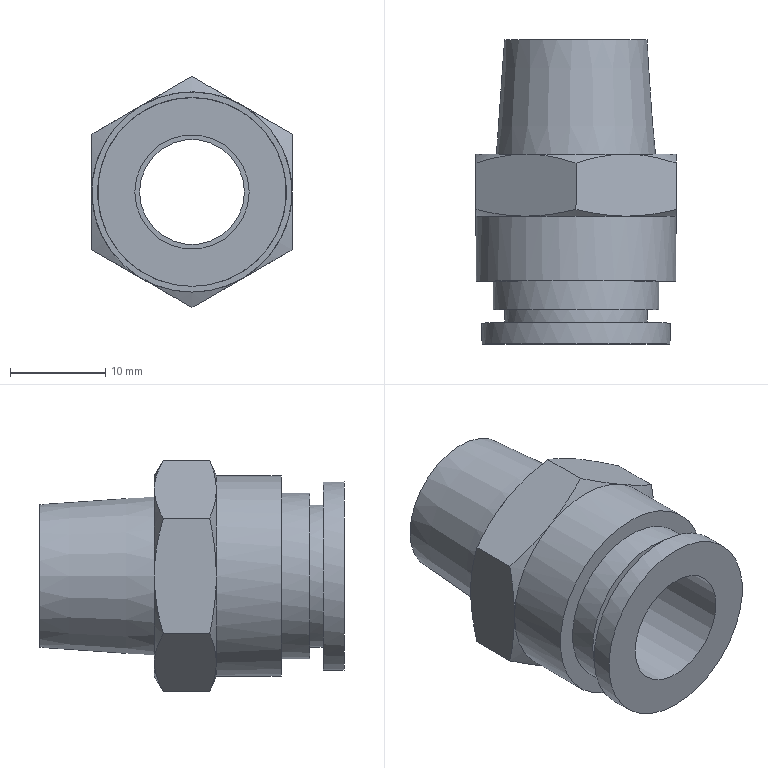Part | STEP file | 1_id114_xmt_txt | 1 solid | 32 faces | box 21 x 31.9 x 24.249 mm | volume 5376 mm3 | plane 13 | cone 13 | cylinder 6 | commonest cylinder face diameters 11 x1 12 x1 15 x1 17.4 x1 19.8 x1 21 x1
STEP:
#1=CARTESIAN_POINT('',(-25.5,-148.,61.));
#2=VERTEX_POINT('',#1);
#3=CARTESIAN_POINT('',(-18.,-148.,61.));
#4=DIRECTION('',(0.,-1.,0.));
#5=DIRECTION('',(-1.,0.,0.));
#6=AXIS2_PLACEMENT_3D('',#3,#4,#5);
#7=CIRCLE('',#6,7.5);
#8=EDGE_CURVE('',#2,#2,#7,.T.);
#9=ORIENTED_EDGE('',*,*,#8,.F.);
#10=EDGE_LOOP('',(#9));
#11=FACE_BOUND('',#10,.T.);
#12=CARTESIAN_POINT('',(-23.5,-148.,61.));
#13=VERTEX_POINT('',#12);
#14=CARTESIAN_POINT('',(-18.,-148.,61.));
#15=DIRECTION('',(0.,1.,0.));
#16=DIRECTION('',(-1.,0.,0.));
#17=AXIS2_PLACEMENT_3D('',#14,#15,#16);
#18=CIRCLE('',#17,5.5);
#19=EDGE_CURVE('',#13,#13,#18,.T.);
#20=ORIENTED_EDGE('',*,*,#19,.F.);
#21=EDGE_LOOP('',(#20));
#22=FACE_BOUND('',#21,.T.);
#23=CARTESIAN_POINT('',(-18.,-148.,61.));
#24=DIRECTION('',(0.,-1.,0.));
#25=DIRECTION('',(0.,0.,-1.));
#26=AXIS2_PLACEMENT_3D('',#23,#24,#25);
#27=PLANE('',#26);
#28=ADVANCED_FACE('',(#11,#22),#27,.F.);
#29=CARTESIAN_POINT('',(-9.65,-160.,61.));
#30=VERTEX_POINT('',#29);
#31=CARTESIAN_POINT('',(-18.,-160.,61.));
#32=DIRECTION('',(0.,-1.,0.));
#33=DIRECTION('',(1.,0.,0.));
#34=AXIS2_PLACEMENT_3D('',#31,#32,#33);
#35=CIRCLE('',#34,8.35);
#36=EDGE_CURVE('',#30,#30,#35,.T.);
#37=ORIENTED_EDGE('',*,*,#36,.F.);
#38=EDGE_LOOP('',(#37));
#39=FACE_BOUND('',#38,.T.);
#40=ORIENTED_EDGE('',*,*,#8,.T.);
#41=EDGE_LOOP('',(#40));
#42=FACE_BOUND('',#41,.T.);
#43=CARTESIAN_POINT('',(-18.,-154.,61.));
#44=DIRECTION('',(0.,-1.,0.));
#45=DIRECTION('',(-1.,0.,0.));
#46=AXIS2_PLACEMENT_3D('',#43,#44,#45);
#47=CONICAL_SURFACE('',#46,7.925,4.052);
#48=ADVANCED_FACE('',(#39,#42),#47,.T.);
#49=CARTESIAN_POINT('',(-23.25,-160.,70.093));
#50=VERTEX_POINT('',#49);
#51=CARTESIAN_POINT('',(-12.75,-160.,70.093));
#52=VERTEX_POINT('',#51);
#53=CARTESIAN_POINT('',(-18.,-160.,61.));
#54=DIRECTION('',(0.,1.,0.));
#55=DIRECTION('',(-0.5,0.,0.866));
#56=AXIS2_PLACEMENT_3D('',#53,#54,#55);
#57=CIRCLE('',#56,10.5);
#58=EDGE_CURVE('',#50,#52,#57,.T.);
#59=ORIENTED_EDGE('',*,*,#58,.T.);
#60=CARTESIAN_POINT('',(-7.5,-160.,61.));
#61=VERTEX_POINT('',#60);
#62=CARTESIAN_POINT('',(-18.,-160.,61.));
#63=DIRECTION('',(0.,1.,0.));
#64=DIRECTION('',(0.5,0.,0.866));
#65=AXIS2_PLACEMENT_3D('',#62,#63,#64);
#66=CIRCLE('',#65,10.5);
#67=EDGE_CURVE('',#52,#61,#66,.T.);
#68=ORIENTED_EDGE('',*,*,#67,.T.);
#69=CARTESIAN_POINT('',(-12.75,-160.,51.907));
#70=VERTEX_POINT('',#69);
#71=CARTESIAN_POINT('',(-18.,-160.,61.));
#72=DIRECTION('',(0.,1.,0.));
#73=DIRECTION('',(1.,0.,0.));
#74=AXIS2_PLACEMENT_3D('',#71,#72,#73);
#75=CIRCLE('',#74,10.5);
#76=EDGE_CURVE('',#61,#70,#75,.T.);
#77=ORIENTED_EDGE('',*,*,#76,.T.);
#78=CARTESIAN_POINT('',(-23.25,-160.,51.907));
#79=VERTEX_POINT('',#78);
#80=CARTESIAN_POINT('',(-18.,-160.,61.));
#81=DIRECTION('',(0.,1.,0.));
#82=DIRECTION('',(0.5,0.,-0.866));
#83=AXIS2_PLACEMENT_3D('',#80,#81,#82);
#84=CIRCLE('',#83,10.5);
#85=EDGE_CURVE('',#70,#79,#84,.T.);
#86=ORIENTED_EDGE('',*,*,#85,.T.);
#87=CARTESIAN_POINT('',(-28.5,-160.,61.));
#88=VERTEX_POINT('',#87);
#89=CARTESIAN_POINT('',(-18.,-160.,61.));
#90=DIRECTION('',(0.,1.,0.));
#91=DIRECTION('',(-0.5,0.,-0.866));
#92=AXIS2_PLACEMENT_3D('',#89,#90,#91);
#93=CIRCLE('',#92,10.5);
#94=EDGE_CURVE('',#79,#88,#93,.T.);
#95=ORIENTED_EDGE('',*,*,#94,.T.);
#96=CARTESIAN_POINT('',(-18.,-160.,61.));
#97=DIRECTION('',(0.,1.,0.));
#98=DIRECTION('',(-1.,0.,0.));
#99=AXIS2_PLACEMENT_3D('',#96,#97,#98);
#100=CIRCLE('',#99,10.5);
#101=EDGE_CURVE('',#88,#50,#100,.T.);
#102=ORIENTED_EDGE('',*,*,#101,.T.);
#103=EDGE_LOOP('',(#59,#68,#77,#86,#95,#102));
#104=FACE_BOUND('',#103,.T.);
#105=ORIENTED_EDGE('',*,*,#36,.T.);
#106=EDGE_LOOP('',(#105));
#107=FACE_BOUND('',#106,.T.);
#108=CARTESIAN_POINT('',(-18.,-160.,61.));
#109=DIRECTION('',(0.,-1.,0.));
#110=DIRECTION('',(0.,0.,-1.));
#111=AXIS2_PLACEMENT_3D('',#108,#109,#110);
#112=PLANE('',#111);
#113=ADVANCED_FACE('',(#104,#107),#112,.F.);
#114=ORIENTED_EDGE('',*,*,#101,.F.);
#115=CARTESIAN_POINT('',(-28.5,-160.938,67.062));
#116=VERTEX_POINT('',#115);
#117=CARTESIAN_POINT('',(-28.5,-160.,61.));
#118=CARTESIAN_POINT('',(-28.5,-160.,63.069));
#119=CARTESIAN_POINT('',(-28.5,-160.366,65.082));
#120=CARTESIAN_POINT('',(-28.5,-160.938,67.062));
#121=B_SPLINE_CURVE_WITH_KNOTS('',3,(#117,#118,#119,#120),.UNSPECIFIED.,.F.,.F.,(4,4),(0.,1.),.UNSPECIFIED.);
#122=EDGE_CURVE('',#88,#116,#121,.T.);
#123=ORIENTED_EDGE('',*,*,#122,.T.);
#124=CARTESIAN_POINT('',(-28.5,-160.938,67.062));
#125=CARTESIAN_POINT('',(-26.785,-160.366,68.052));
#126=CARTESIAN_POINT('',(-25.042,-160.,69.059));
#127=CARTESIAN_POINT('',(-23.25,-160.,70.093));
#128=B_SPLINE_CURVE_WITH_KNOTS('',3,(#124,#125,#126,#127),.UNSPECIFIED.,.F.,.F.,(4,4),(0.,1.),.UNSPECIFIED.);
#129=EDGE_CURVE('',#116,#50,#128,.T.);
#130=ORIENTED_EDGE('',*,*,#129,.T.);
#131=EDGE_LOOP('',(#114,#123,#130));
#132=FACE_OUTER_BOUND('',#131,.T.);
#133=CARTESIAN_POINT('',(-18.,-160.469,61.));
#134=DIRECTION('',(0.,-1.,0.));
#135=DIRECTION('',(-1.,0.,0.));
#136=AXIS2_PLACEMENT_3D('',#133,#134,#135);
#137=CONICAL_SURFACE('',#136,11.312,60.);
#138=ADVANCED_FACE('',(#132),#137,.T.);
#139=ORIENTED_EDGE('',*,*,#58,.F.);
#140=CARTESIAN_POINT('',(-18.,-160.938,73.124));
#141=VERTEX_POINT('',#140);
#142=CARTESIAN_POINT('',(-23.25,-160.,70.093));
#143=CARTESIAN_POINT('',(-21.458,-160.,71.128));
#144=CARTESIAN_POINT('',(-19.715,-160.366,72.134));
#145=CARTESIAN_POINT('',(-18.,-160.938,73.124));
#146=B_SPLINE_CURVE_WITH_KNOTS('',3,(#142,#143,#144,#145),.UNSPECIFIED.,.F.,.F.,(4,4),(0.,1.),.UNSPECIFIED.);
#147=EDGE_CURVE('',#50,#141,#146,.T.);
#148=ORIENTED_EDGE('',*,*,#147,.T.);
#149=CARTESIAN_POINT('',(-18.,-160.938,73.124));
#150=CARTESIAN_POINT('',(-16.285,-160.366,72.134));
#151=CARTESIAN_POINT('',(-14.542,-160.,71.128));
#152=CARTESIAN_POINT('',(-12.75,-160.,70.093));
#153=B_SPLINE_CURVE_WITH_KNOTS('',3,(#149,#150,#151,#152),.UNSPECIFIED.,.F.,.F.,(4,4),(0.,1.),.UNSPECIFIED.);
#154=EDGE_CURVE('',#141,#52,#153,.T.);
#155=ORIENTED_EDGE('',*,*,#154,.T.);
#156=EDGE_LOOP('',(#139,#148,#155));
#157=FACE_OUTER_BOUND('',#156,.T.);
#158=CARTESIAN_POINT('',(-18.,-160.469,61.));
#159=DIRECTION('',(0.,-1.,0.));
#160=DIRECTION('',(-1.,0.,0.));
#161=AXIS2_PLACEMENT_3D('',#158,#159,#160);
#162=CONICAL_SURFACE('',#161,11.312,60.);
#163=ADVANCED_FACE('',(#157),#162,.T.);
#164=ORIENTED_EDGE('',*,*,#67,.F.);
#165=CARTESIAN_POINT('',(-7.5,-160.938,67.062));
#166=VERTEX_POINT('',#165);
#167=CARTESIAN_POINT('',(-12.75,-160.,70.093));
#168=CARTESIAN_POINT('',(-10.958,-160.,69.059));
#169=CARTESIAN_POINT('',(-9.215,-160.366,68.052));
#170=CARTESIAN_POINT('',(-7.5,-160.938,67.062));
#171=B_SPLINE_CURVE_WITH_KNOTS('',3,(#167,#168,#169,#170),.UNSPECIFIED.,.F.,.F.,(4,4),(0.,1.),.UNSPECIFIED.);
#172=EDGE_CURVE('',#52,#166,#171,.T.);
#173=ORIENTED_EDGE('',*,*,#172,.T.);
#174=CARTESIAN_POINT('',(-7.5,-160.938,67.062));
#175=CARTESIAN_POINT('',(-7.5,-160.366,65.082));
#176=CARTESIAN_POINT('',(-7.5,-160.,63.069));
#177=CARTESIAN_POINT('',(-7.5,-160.,61.));
#178=B_SPLINE_CURVE_WITH_KNOTS('',3,(#174,#175,#176,#177),.UNSPECIFIED.,.F.,.F.,(4,4),(0.,1.),.UNSPECIFIED.);
#179=EDGE_CURVE('',#166,#61,#178,.T.);
#180=ORIENTED_EDGE('',*,*,#179,.T.);
#181=EDGE_LOOP('',(#164,#173,#180));
#182=FACE_OUTER_BOUND('',#181,.T.);
#183=CARTESIAN_POINT('',(-18.,-160.469,61.));
#184=DIRECTION('',(0.,-1.,0.));
#185=DIRECTION('',(-1.,0.,0.));
#186=AXIS2_PLACEMENT_3D('',#183,#184,#185);
#187=CONICAL_SURFACE('',#186,11.312,60.);
#188=ADVANCED_FACE('',(#182),#187,.T.);
#189=CARTESIAN_POINT('',(-18.,-165.798,73.124));
#190=VERTEX_POINT('',#189);
#191=CARTESIAN_POINT('',(-18.,-160.938,73.124));
#192=DIRECTION('',(0.,-1.,0.));
#193=VECTOR('',#192,1.);
#194=LINE('',#191,#193);
#195=EDGE_CURVE('',#141,#190,#194,.T.);
#196=ORIENTED_EDGE('',*,*,#195,.F.);
#197=ORIENTED_EDGE('',*,*,#147,.F.);
#198=ORIENTED_EDGE('',*,*,#129,.F.);
#199=CARTESIAN_POINT('',(-28.5,-165.798,67.062));
#200=VERTEX_POINT('',#199);
#201=CARTESIAN_POINT('',(-28.5,-160.938,67.062));
#202=DIRECTION('',(0.,-1.,0.));
#203=VECTOR('',#202,1.);
#204=LINE('',#201,#203);
#205=EDGE_CURVE('',#116,#200,#204,.T.);
#206=ORIENTED_EDGE('',*,*,#205,.T.);
#207=CARTESIAN_POINT('',(-23.25,-166.5,70.093));
#208=VERTEX_POINT('',#207);
#209=CARTESIAN_POINT('',(-23.25,-166.5,70.093));
#210=CARTESIAN_POINT('',(-25.023,-166.5,69.069));
#211=CARTESIAN_POINT('',(-26.77,-166.23,68.061));
#212=CARTESIAN_POINT('',(-28.5,-165.798,67.062));
#213=B_SPLINE_CURVE_WITH_KNOTS('',3,(#209,#210,#211,#212),.UNSPECIFIED.,.F.,.F.,(4,4),(0.,1.),.UNSPECIFIED.);
#214=EDGE_CURVE('',#208,#200,#213,.T.);
#215=ORIENTED_EDGE('',*,*,#214,.F.);
#216=CARTESIAN_POINT('',(-18.,-165.798,73.124));
#217=CARTESIAN_POINT('',(-19.73,-166.23,72.125));
#218=CARTESIAN_POINT('',(-21.477,-166.5,71.117));
#219=CARTESIAN_POINT('',(-23.25,-166.5,70.093));
#220=B_SPLINE_CURVE_WITH_KNOTS('',3,(#216,#217,#218,#219),.UNSPECIFIED.,.F.,.F.,(4,4),(0.,1.),.UNSPECIFIED.);
#221=EDGE_CURVE('',#190,#208,#220,.T.);
#222=ORIENTED_EDGE('',*,*,#221,.F.);
#223=EDGE_LOOP('',(#196,#197,#198,#206,#215,#222));
#224=FACE_OUTER_BOUND('',#223,.T.);
#225=CARTESIAN_POINT('',(-18.,-160.,73.124));
#226=DIRECTION('',(-0.5,0.,0.866));
#227=DIRECTION('',(0.866,0.,0.5));
#228=AXIS2_PLACEMENT_3D('',#225,#226,#227);
#229=PLANE('',#228);
#230=ADVANCED_FACE('',(#224),#229,.T.);
#231=CARTESIAN_POINT('',(-7.5,-166.5,61.));
#232=VERTEX_POINT('',#231);
#233=CARTESIAN_POINT('',(-7.5,-165.798,67.062));
#234=VERTEX_POINT('',#233);
#235=CARTESIAN_POINT('',(-7.5,-166.5,61.));
#236=CARTESIAN_POINT('',(-7.5,-166.5,63.048));
#237=CARTESIAN_POINT('',(-7.5,-166.23,65.064));
#238=CARTESIAN_POINT('',(-7.5,-165.798,67.062));
#239=B_SPLINE_CURVE_WITH_KNOTS('',3,(#235,#236,#237,#238),.UNSPECIFIED.,.F.,.F.,(4,4),(0.,1.),.UNSPECIFIED.);
#240=EDGE_CURVE('',#232,#234,#239,.T.);
#241=ORIENTED_EDGE('',*,*,#240,.T.);
#242=CARTESIAN_POINT('',(-12.75,-166.5,70.093));
#243=VERTEX_POINT('',#242);
#244=CARTESIAN_POINT('',(-7.5,-165.798,67.062));
#245=CARTESIAN_POINT('',(-9.23,-166.23,68.061));
#246=CARTESIAN_POINT('',(-10.977,-166.5,69.069));
#247=CARTESIAN_POINT('',(-12.75,-166.5,70.093));
#248=B_SPLINE_CURVE_WITH_KNOTS('',3,(#244,#245,#246,#247),.UNSPECIFIED.,.F.,.F.,(4,4),(0.,1.),.UNSPECIFIED.);
#249=EDGE_CURVE('',#234,#243,#248,.T.);
#250=ORIENTED_EDGE('',*,*,#249,.T.);
#251=CARTESIAN_POINT('',(-18.,-166.5,61.));
#252=DIRECTION('',(0.,-1.,0.));
#253=DIRECTION('',(1.,0.,0.));
#254=AXIS2_PLACEMENT_3D('',#251,#252,#253);
#255=CIRCLE('',#254,10.5);
#256=EDGE_CURVE('',#232,#243,#255,.T.);
#257=ORIENTED_EDGE('',*,*,#256,.F.);
#258=EDGE_LOOP('',(#241,#250,#257));
#259=FACE_OUTER_BOUND('',#258,.T.);
#260=CARTESIAN_POINT('',(-18.,-166.149,61.));
#261=DIRECTION('',(0.,1.,0.));
#262=DIRECTION('',(1.,0.,0.));
#263=AXIS2_PLACEMENT_3D('',#260,#261,#262);
#264=CONICAL_SURFACE('',#263,11.312,66.635);
#265=ADVANCED_FACE('',(#259),#264,.T.);
#266=CARTESIAN_POINT('',(-12.75,-166.5,70.093));
#267=CARTESIAN_POINT('',(-14.523,-166.5,71.117));
#268=CARTESIAN_POINT('',(-16.27,-166.23,72.125));
#269=CARTESIAN_POINT('',(-18.,-165.798,73.124));
#270=B_SPLINE_CURVE_WITH_KNOTS('',3,(#266,#267,#268,#269),.UNSPECIFIED.,.F.,.F.,(4,4),(0.,1.),.UNSPECIFIED.);
#271=EDGE_CURVE('',#243,#190,#270,.T.);
#272=ORIENTED_EDGE('',*,*,#271,.T.);
#273=ORIENTED_EDGE('',*,*,#221,.T.);
#274=CARTESIAN_POINT('',(-18.,-166.5,61.));
#275=DIRECTION('',(0.,-1.,0.));
#276=DIRECTION('',(0.,0.,1.));
#277=AXIS2_PLACEMENT_3D('',#274,#275,#276);
#278=CIRCLE('',#277,10.5);
#279=EDGE_CURVE('',#243,#208,#278,.T.);
#280=ORIENTED_EDGE('',*,*,#279,.F.);
#281=EDGE_LOOP('',(#272,#273,#280));
#282=FACE_OUTER_BOUND('',#281,.T.);
#283=CARTESIAN_POINT('',(-18.,-166.149,61.));
#284=DIRECTION('',(0.,1.,0.));
#285=DIRECTION('',(1.,0.,0.));
#286=AXIS2_PLACEMENT_3D('',#283,#284,#285);
#287=CONICAL_SURFACE('',#286,11.312,66.635);
#288=ADVANCED_FACE('',(#282),#287,.T.);
#289=ORIENTED_EDGE('',*,*,#214,.T.);
#290=CARTESIAN_POINT('',(-28.5,-166.5,61.));
#291=VERTEX_POINT('',#290);
#292=CARTESIAN_POINT('',(-28.5,-165.798,67.062));
#293=CARTESIAN_POINT('',(-28.5,-166.23,65.064));
#294=CARTESIAN_POINT('',(-28.5,-166.5,63.048));
#295=CARTESIAN_POINT('',(-28.5,-166.5,61.));
#296=B_SPLINE_CURVE_WITH_KNOTS('',3,(#292,#293,#294,#295),.UNSPECIFIED.,.F.,.F.,(4,4),(0.,1.),.UNSPECIFIED.);
#297=EDGE_CURVE('',#200,#291,#296,.T.);
#298=ORIENTED_EDGE('',*,*,#297,.T.);
#299=CARTESIAN_POINT('',(-18.,-166.5,61.));
#300=DIRECTION('',(0.,-1.,0.));
#301=DIRECTION('',(-0.5,0.,0.866));
#302=AXIS2_PLACEMENT_3D('',#299,#300,#301);
#303=CIRCLE('',#302,10.5);
#304=EDGE_CURVE('',#208,#291,#303,.T.);
#305=ORIENTED_EDGE('',*,*,#304,.F.);
#306=EDGE_LOOP('',(#289,#298,#305));
#307=FACE_OUTER_BOUND('',#306,.T.);
#308=CARTESIAN_POINT('',(-18.,-166.149,61.));
#309=DIRECTION('',(0.,1.,0.));
#310=DIRECTION('',(1.,0.,0.));
#311=AXIS2_PLACEMENT_3D('',#308,#309,#310);
#312=CONICAL_SURFACE('',#311,11.312,66.635);
#313=ADVANCED_FACE('',(#307),#312,.T.);
#314=CARTESIAN_POINT('',(-18.,-173.3,50.5));
#315=VERTEX_POINT('',#314);
#316=CARTESIAN_POINT('',(-18.,-173.3,61.));
#317=DIRECTION('',(0.,-1.,0.));
#318=DIRECTION('',(0.,0.,-1.));
#319=AXIS2_PLACEMENT_3D('',#316,#317,#318);
#320=CIRCLE('',#319,10.5);
#321=EDGE_CURVE('',#315,#315,#320,.T.);
#322=ORIENTED_EDGE('',*,*,#321,.F.);
#323=EDGE_LOOP('',(#322));
#324=FACE_BOUND('',#323,.T.);
#325=CARTESIAN_POINT('',(-12.75,-166.5,51.907));
#326=VERTEX_POINT('',#325);
#327=CARTESIAN_POINT('',(-18.,-166.5,61.));
#328=DIRECTION('',(0.,-1.,0.));
#329=DIRECTION('',(0.5,0.,-0.866));
#330=AXIS2_PLACEMENT_3D('',#327,#328,#329);
#331=CIRCLE('',#330,10.5);
#332=EDGE_CURVE('',#326,#232,#331,.T.);
#333=ORIENTED_EDGE('',*,*,#332,.T.);
#334=ORIENTED_EDGE('',*,*,#256,.T.);
#335=ORIENTED_EDGE('',*,*,#279,.T.);
#336=ORIENTED_EDGE('',*,*,#304,.T.);
#337=CARTESIAN_POINT('',(-23.25,-166.5,51.907));
#338=VERTEX_POINT('',#337);
#339=CARTESIAN_POINT('',(-18.,-166.5,61.));
#340=DIRECTION('',(0.,-1.,0.));
#341=DIRECTION('',(-1.,0.,0.));
#342=AXIS2_PLACEMENT_3D('',#339,#340,#341);
#343=CIRCLE('',#342,10.5);
#344=EDGE_CURVE('',#291,#338,#343,.T.);
#345=ORIENTED_EDGE('',*,*,#344,.T.);
#346=CARTESIAN_POINT('',(-18.,-166.5,61.));
#347=DIRECTION('',(0.,-1.,0.));
#348=DIRECTION('',(0.,0.,-1.));
#349=AXIS2_PLACEMENT_3D('',#346,#347,#348);
#350=CIRCLE('',#349,10.5);
#351=EDGE_CURVE('',#338,#326,#350,.T.);
#352=ORIENTED_EDGE('',*,*,#351,.T.);
#353=EDGE_LOOP('',(#333,#334,#335,#336,#345,#352));
#354=FACE_BOUND('',#353,.T.);
#355=CARTESIAN_POINT('',(-18.,-166.5,61.));
#356=DIRECTION('',(0.,1.,0.));
#357=DIRECTION('',(0.,0.,1.));
#358=AXIS2_PLACEMENT_3D('',#355,#356,#357);
#359=CYLINDRICAL_SURFACE('',#358,10.5);
#360=ADVANCED_FACE('',(#324,#354),#359,.T.);
#361=ORIENTED_EDGE('',*,*,#351,.F.);
#362=CARTESIAN_POINT('',(-18.,-165.798,48.876));
#363=VERTEX_POINT('',#362);
#364=CARTESIAN_POINT('',(-23.25,-166.5,51.907));
#365=CARTESIAN_POINT('',(-21.477,-166.5,50.883));
#366=CARTESIAN_POINT('',(-19.73,-166.23,49.875));
#367=CARTESIAN_POINT('',(-18.,-165.798,48.876));
#368=B_SPLINE_CURVE_WITH_KNOTS('',3,(#364,#365,#366,#367),.UNSPECIFIED.,.F.,.F.,(4,4),(0.,1.),.UNSPECIFIED.);
#369=EDGE_CURVE('',#338,#363,#368,.T.);
#370=ORIENTED_EDGE('',*,*,#369,.T.);
#371=CARTESIAN_POINT('',(-18.,-165.798,48.876));
#372=CARTESIAN_POINT('',(-16.27,-166.23,49.875));
#373=CARTESIAN_POINT('',(-14.523,-166.5,50.883));
#374=CARTESIAN_POINT('',(-12.75,-166.5,51.907));
#375=B_SPLINE_CURVE_WITH_KNOTS('',3,(#371,#372,#373,#374),.UNSPECIFIED.,.F.,.F.,(4,4),(0.,1.),.UNSPECIFIED.);
#376=EDGE_CURVE('',#363,#326,#375,.T.);
#377=ORIENTED_EDGE('',*,*,#376,.T.);
#378=EDGE_LOOP('',(#361,#370,#377));
#379=FACE_OUTER_BOUND('',#378,.T.);
#380=CARTESIAN_POINT('',(-18.,-166.149,61.));
#381=DIRECTION('',(0.,1.,0.));
#382=DIRECTION('',(1.,0.,0.));
#383=AXIS2_PLACEMENT_3D('',#380,#381,#382);
#384=CONICAL_SURFACE('',#383,11.312,66.635);
#385=ADVANCED_FACE('',(#379),#384,.T.);
#386=CARTESIAN_POINT('',(-7.5,-165.798,54.938));
#387=VERTEX_POINT('',#386);
#388=CARTESIAN_POINT('',(-12.75,-166.5,51.907));
#389=CARTESIAN_POINT('',(-10.977,-166.5,52.931));
#390=CARTESIAN_POINT('',(-9.23,-166.23,53.939));
#391=CARTESIAN_POINT('',(-7.5,-165.798,54.938));
#392=B_SPLINE_CURVE_WITH_KNOTS('',3,(#388,#389,#390,#391),.UNSPECIFIED.,.F.,.F.,(4,4),(0.,1.),.UNSPECIFIED.);
#393=EDGE_CURVE('',#326,#387,#392,.T.);
#394=ORIENTED_EDGE('',*,*,#393,.T.);
#395=CARTESIAN_POINT('',(-7.5,-165.798,54.938));
#396=CARTESIAN_POINT('',(-7.5,-166.23,56.936));
#397=CARTESIAN_POINT('',(-7.5,-166.5,58.952));
#398=CARTESIAN_POINT('',(-7.5,-166.5,61.));
#399=B_SPLINE_CURVE_WITH_KNOTS('',3,(#395,#396,#397,#398),.UNSPECIFIED.,.F.,.F.,(4,4),(0.,1.),.UNSPECIFIED.);
#400=EDGE_CURVE('',#387,#232,#399,.T.);
#401=ORIENTED_EDGE('',*,*,#400,.T.);
#402=ORIENTED_EDGE('',*,*,#332,.F.);
#403=EDGE_LOOP('',(#394,#401,#402));
#404=FACE_OUTER_BOUND('',#403,.T.);
#405=CARTESIAN_POINT('',(-18.,-166.149,61.));
#406=DIRECTION('',(0.,1.,0.));
#407=DIRECTION('',(1.,0.,0.));
#408=AXIS2_PLACEMENT_3D('',#405,#406,#407);
#409=CONICAL_SURFACE('',#408,11.312,66.635);
#410=ADVANCED_FACE('',(#404),#409,.T.);
#411=CARTESIAN_POINT('',(-28.5,-165.798,54.938));
#412=VERTEX_POINT('',#411);
#413=CARTESIAN_POINT('',(-28.5,-166.5,61.));
#414=CARTESIAN_POINT('',(-28.5,-166.5,58.952));
#415=CARTESIAN_POINT('',(-28.5,-166.23,56.936));
#416=CARTESIAN_POINT('',(-28.5,-165.798,54.938));
#417=B_SPLINE_CURVE_WITH_KNOTS('',3,(#413,#414,#415,#416),.UNSPECIFIED.,.F.,.F.,(4,4),(0.,1.),.UNSPECIFIED.);
#418=EDGE_CURVE('',#291,#412,#417,.T.);
#419=ORIENTED_EDGE('',*,*,#418,.T.);
#420=CARTESIAN_POINT('',(-28.5,-165.798,54.938));
#421=CARTESIAN_POINT('',(-26.77,-166.23,53.939));
#422=CARTESIAN_POINT('',(-25.023,-166.5,52.931));
#423=CARTESIAN_POINT('',(-23.25,-166.5,51.907));
#424=B_SPLINE_CURVE_WITH_KNOTS('',3,(#420,#421,#422,#423),.UNSPECIFIED.,.F.,.F.,(4,4),(0.,1.),.UNSPECIFIED.);
#425=EDGE_CURVE('',#412,#338,#424,.T.);
#426=ORIENTED_EDGE('',*,*,#425,.T.);
#427=ORIENTED_EDGE('',*,*,#344,.F.);
#428=EDGE_LOOP('',(#419,#426,#427));
#429=FACE_OUTER_BOUND('',#428,.T.);
#430=CARTESIAN_POINT('',(-18.,-166.149,61.));
#431=DIRECTION('',(0.,1.,0.));
#432=DIRECTION('',(1.,0.,0.));
#433=AXIS2_PLACEMENT_3D('',#430,#431,#432);
#434=CONICAL_SURFACE('',#433,11.312,66.635);
#435=ADVANCED_FACE('',(#429),#434,.T.);
#436=CARTESIAN_POINT('',(-18.,-160.938,48.876));
#437=VERTEX_POINT('',#436);
#438=CARTESIAN_POINT('',(-18.,-160.938,48.876));
#439=DIRECTION('',(0.,-1.,0.));
#440=VECTOR('',#439,1.);
#441=LINE('',#438,#440);
#442=EDGE_CURVE('',#437,#363,#441,.T.);
#443=ORIENTED_EDGE('',*,*,#442,.F.);
#444=CARTESIAN_POINT('',(-12.75,-160.,51.907));
#445=CARTESIAN_POINT('',(-14.542,-160.,50.872));
#446=CARTESIAN_POINT('',(-16.285,-160.366,49.866));
#447=CARTESIAN_POINT('',(-18.,-160.938,48.876));
#448=B_SPLINE_CURVE_WITH_KNOTS('',3,(#444,#445,#446,#447),.UNSPECIFIED.,.F.,.F.,(4,4),(0.,1.),.UNSPECIFIED.);
#449=EDGE_CURVE('',#70,#437,#448,.T.);
#450=ORIENTED_EDGE('',*,*,#449,.F.);
#451=CARTESIAN_POINT('',(-7.5,-160.938,54.938));
#452=VERTEX_POINT('',#451);
#453=CARTESIAN_POINT('',(-7.5,-160.938,54.938));
#454=CARTESIAN_POINT('',(-9.215,-160.366,53.948));
#455=CARTESIAN_POINT('',(-10.958,-160.,52.941));
#456=CARTESIAN_POINT('',(-12.75,-160.,51.907));
#457=B_SPLINE_CURVE_WITH_KNOTS('',3,(#453,#454,#455,#456),.UNSPECIFIED.,.F.,.F.,(4,4),(0.,1.),.UNSPECIFIED.);
#458=EDGE_CURVE('',#452,#70,#457,.T.);
#459=ORIENTED_EDGE('',*,*,#458,.F.);
#460=CARTESIAN_POINT('',(-7.5,-160.938,54.938));
#461=DIRECTION('',(0.,-1.,0.));
#462=VECTOR('',#461,1.);
#463=LINE('',#460,#462);
#464=EDGE_CURVE('',#452,#387,#463,.T.);
#465=ORIENTED_EDGE('',*,*,#464,.T.);
#466=ORIENTED_EDGE('',*,*,#393,.F.);
#467=ORIENTED_EDGE('',*,*,#376,.F.);
#468=EDGE_LOOP('',(#443,#450,#459,#465,#466,#467));
#469=FACE_OUTER_BOUND('',#468,.T.);
#470=CARTESIAN_POINT('',(-18.,-160.,48.876));
#471=DIRECTION('',(0.5,0.,-0.866));
#472=DIRECTION('',(0.,1.,0.));
#473=AXIS2_PLACEMENT_3D('',#470,#471,#472);
#474=PLANE('',#473);
#475=ADVANCED_FACE('',(#469),#474,.T.);
#476=ORIENTED_EDGE('',*,*,#464,.F.);
#477=CARTESIAN_POINT('',(-7.5,-160.,61.));
#478=CARTESIAN_POINT('',(-7.5,-160.,58.931));
#479=CARTESIAN_POINT('',(-7.5,-160.366,56.918));
#480=CARTESIAN_POINT('',(-7.5,-160.938,54.938));
#481=B_SPLINE_CURVE_WITH_KNOTS('',3,(#477,#478,#479,#480),.UNSPECIFIED.,.F.,.F.,(4,4),(0.,1.),.UNSPECIFIED.);
#482=EDGE_CURVE('',#61,#452,#481,.T.);
#483=ORIENTED_EDGE('',*,*,#482,.F.);
#484=ORIENTED_EDGE('',*,*,#179,.F.);
#485=CARTESIAN_POINT('',(-7.5,-160.938,67.062));
#486=DIRECTION('',(0.,-1.,0.));
#487=VECTOR('',#486,1.);
#488=LINE('',#485,#487);
#489=EDGE_CURVE('',#166,#234,#488,.T.);
#490=ORIENTED_EDGE('',*,*,#489,.T.);
#491=ORIENTED_EDGE('',*,*,#240,.F.);
#492=ORIENTED_EDGE('',*,*,#400,.F.);
#493=EDGE_LOOP('',(#476,#483,#484,#490,#491,#492));
#494=FACE_OUTER_BOUND('',#493,.T.);
#495=CARTESIAN_POINT('',(-7.5,-160.,54.938));
#496=DIRECTION('',(1.,0.,0.));
#497=DIRECTION('',(0.,0.,1.));
#498=AXIS2_PLACEMENT_3D('',#495,#496,#497);
#499=PLANE('',#498);
#500=ADVANCED_FACE('',(#494),#499,.T.);
#501=ORIENTED_EDGE('',*,*,#489,.F.);
#502=ORIENTED_EDGE('',*,*,#172,.F.);
#503=ORIENTED_EDGE('',*,*,#154,.F.);
#504=ORIENTED_EDGE('',*,*,#195,.T.);
#505=ORIENTED_EDGE('',*,*,#271,.F.);
#506=ORIENTED_EDGE('',*,*,#249,.F.);
#507=EDGE_LOOP('',(#501,#502,#503,#504,#505,#506));
#508=FACE_OUTER_BOUND('',#507,.T.);
#509=CARTESIAN_POINT('',(-7.5,-160.,67.062));
#510=DIRECTION('',(0.5,0.,0.866));
#511=DIRECTION('',(0.,1.,0.));
#512=AXIS2_PLACEMENT_3D('',#509,#510,#511);
#513=PLANE('',#512);
#514=ADVANCED_FACE('',(#508),#513,.T.);
#515=ORIENTED_EDGE('',*,*,#76,.F.);
#516=ORIENTED_EDGE('',*,*,#482,.T.);
#517=ORIENTED_EDGE('',*,*,#458,.T.);
#518=EDGE_LOOP('',(#515,#516,#517));
#519=FACE_OUTER_BOUND('',#518,.T.);
#520=CARTESIAN_POINT('',(-18.,-160.469,61.));
#521=DIRECTION('',(0.,-1.,0.));
#522=DIRECTION('',(-1.,0.,0.));
#523=AXIS2_PLACEMENT_3D('',#520,#521,#522);
#524=CONICAL_SURFACE('',#523,11.312,60.);
#525=ADVANCED_FACE('',(#519),#524,.T.);
#526=ORIENTED_EDGE('',*,*,#85,.F.);
#527=ORIENTED_EDGE('',*,*,#449,.T.);
#528=CARTESIAN_POINT('',(-18.,-160.938,48.876));
#529=CARTESIAN_POINT('',(-19.715,-160.366,49.866));
#530=CARTESIAN_POINT('',(-21.458,-160.,50.872));
#531=CARTESIAN_POINT('',(-23.25,-160.,51.907));
#532=B_SPLINE_CURVE_WITH_KNOTS('',3,(#528,#529,#530,#531),.UNSPECIFIED.,.F.,.F.,(4,4),(0.,1.),.UNSPECIFIED.);
#533=EDGE_CURVE('',#437,#79,#532,.T.);
#534=ORIENTED_EDGE('',*,*,#533,.T.);
#535=EDGE_LOOP('',(#526,#527,#534));
#536=FACE_OUTER_BOUND('',#535,.T.);
#537=CARTESIAN_POINT('',(-18.,-160.469,61.));
#538=DIRECTION('',(0.,-1.,0.));
#539=DIRECTION('',(-1.,0.,0.));
#540=AXIS2_PLACEMENT_3D('',#537,#538,#539);
#541=CONICAL_SURFACE('',#540,11.312,60.);
#542=ADVANCED_FACE('',(#536),#541,.T.);
#543=ORIENTED_EDGE('',*,*,#94,.F.);
#544=CARTESIAN_POINT('',(-28.5,-160.938,54.938));
#545=VERTEX_POINT('',#544);
#546=CARTESIAN_POINT('',(-23.25,-160.,51.907));
#547=CARTESIAN_POINT('',(-25.042,-160.,52.941));
#548=CARTESIAN_POINT('',(-26.785,-160.366,53.948));
#549=CARTESIAN_POINT('',(-28.5,-160.938,54.938));
#550=B_SPLINE_CURVE_WITH_KNOTS('',3,(#546,#547,#548,#549),.UNSPECIFIED.,.F.,.F.,(4,4),(0.,1.),.UNSPECIFIED.);
#551=EDGE_CURVE('',#79,#545,#550,.T.);
#552=ORIENTED_EDGE('',*,*,#551,.T.);
#553=CARTESIAN_POINT('',(-28.5,-160.938,54.938));
#554=CARTESIAN_POINT('',(-28.5,-160.366,56.918));
#555=CARTESIAN_POINT('',(-28.5,-160.,58.931));
#556=CARTESIAN_POINT('',(-28.5,-160.,61.));
#557=B_SPLINE_CURVE_WITH_KNOTS('',3,(#553,#554,#555,#556),.UNSPECIFIED.,.F.,.F.,(4,4),(0.,1.),.UNSPECIFIED.);
#558=EDGE_CURVE('',#545,#88,#557,.T.);
#559=ORIENTED_EDGE('',*,*,#558,.T.);
#560=EDGE_LOOP('',(#543,#552,#559));
#561=FACE_OUTER_BOUND('',#560,.T.);
#562=CARTESIAN_POINT('',(-18.,-160.469,61.));
#563=DIRECTION('',(0.,-1.,0.));
#564=DIRECTION('',(-1.,0.,0.));
#565=AXIS2_PLACEMENT_3D('',#562,#563,#564);
#566=CONICAL_SURFACE('',#565,11.312,60.);
#567=ADVANCED_FACE('',(#561),#566,.T.);
#568=CARTESIAN_POINT('',(-28.5,-160.938,54.938));
#569=DIRECTION('',(0.,-1.,0.));
#570=VECTOR('',#569,1.);
#571=LINE('',#568,#570);
#572=EDGE_CURVE('',#545,#412,#571,.T.);
#573=ORIENTED_EDGE('',*,*,#572,.F.);
#574=ORIENTED_EDGE('',*,*,#551,.F.);
#575=ORIENTED_EDGE('',*,*,#533,.F.);
#576=ORIENTED_EDGE('',*,*,#442,.T.);
#577=ORIENTED_EDGE('',*,*,#369,.F.);
#578=ORIENTED_EDGE('',*,*,#425,.F.);
#579=EDGE_LOOP('',(#573,#574,#575,#576,#577,#578));
#580=FACE_OUTER_BOUND('',#579,.T.);
#581=CARTESIAN_POINT('',(-28.5,-160.,54.938));
#582=DIRECTION('',(-0.5,0.,-0.866));
#583=DIRECTION('',(0.,-1.,0.));
#584=AXIS2_PLACEMENT_3D('',#581,#582,#583);
#585=PLANE('',#584);
#586=ADVANCED_FACE('',(#580),#585,.T.);
#587=ORIENTED_EDGE('',*,*,#297,.F.);
#588=ORIENTED_EDGE('',*,*,#205,.F.);
#589=ORIENTED_EDGE('',*,*,#122,.F.);
#590=ORIENTED_EDGE('',*,*,#558,.F.);
#591=ORIENTED_EDGE('',*,*,#572,.T.);
#592=ORIENTED_EDGE('',*,*,#418,.F.);
#593=EDGE_LOOP('',(#587,#588,#589,#590,#591,#592));
#594=FACE_OUTER_BOUND('',#593,.T.);
#595=CARTESIAN_POINT('',(-28.5,-160.,67.062));
#596=DIRECTION('',(-1.,0.,0.));
#597=DIRECTION('',(0.,-1.,0.));
#598=AXIS2_PLACEMENT_3D('',#595,#596,#597);
#599=PLANE('',#598);
#600=ADVANCED_FACE('',(#594),#599,.T.);
#601=ORIENTED_EDGE('',*,*,#321,.T.);
#602=EDGE_LOOP('',(#601));
#603=FACE_BOUND('',#602,.T.);
#604=CARTESIAN_POINT('',(-18.,-173.3,52.3));
#605=VERTEX_POINT('',#604);
#606=CARTESIAN_POINT('',(-18.,-173.3,61.));
#607=DIRECTION('',(0.,-1.,0.));
#608=DIRECTION('',(0.,0.,-1.));
#609=AXIS2_PLACEMENT_3D('',#606,#607,#608);
#610=CIRCLE('',#609,8.7);
#611=EDGE_CURVE('',#605,#605,#610,.T.);
#612=ORIENTED_EDGE('',*,*,#611,.F.);
#613=EDGE_LOOP('',(#612));
#614=FACE_BOUND('',#613,.T.);
#615=CARTESIAN_POINT('',(-18.,-173.3,61.));
#616=DIRECTION('',(0.,-1.,0.));
#617=DIRECTION('',(0.,0.,-1.));
#618=AXIS2_PLACEMENT_3D('',#615,#616,#617);
#619=PLANE('',#618);
#620=ADVANCED_FACE('',(#603,#614),#619,.T.);
#621=ORIENTED_EDGE('',*,*,#611,.T.);
#622=EDGE_LOOP('',(#621));
#623=FACE_BOUND('',#622,.T.);
#624=CARTESIAN_POINT('',(-18.,-176.3,69.7));
#625=VERTEX_POINT('',#624);
#626=CARTESIAN_POINT('',(-18.,-176.3,61.));
#627=DIRECTION('',(0.,-1.,0.));
#628=DIRECTION('',(0.,0.,1.));
#629=AXIS2_PLACEMENT_3D('',#626,#627,#628);
#630=CIRCLE('',#629,8.7);
#631=EDGE_CURVE('',#625,#625,#630,.T.);
#632=ORIENTED_EDGE('',*,*,#631,.F.);
#633=EDGE_LOOP('',(#632));
#634=FACE_BOUND('',#633,.T.);
#635=CARTESIAN_POINT('',(-18.,-173.3,61.));
#636=DIRECTION('',(0.,1.,0.));
#637=DIRECTION('',(0.,0.,-1.));
#638=AXIS2_PLACEMENT_3D('',#635,#636,#637);
#639=CYLINDRICAL_SURFACE('',#638,8.7);
#640=ADVANCED_FACE('',(#623,#634),#639,.T.);
#641=ORIENTED_EDGE('',*,*,#631,.T.);
#642=EDGE_LOOP('',(#641));
#643=FACE_BOUND('',#642,.T.);
#644=CARTESIAN_POINT('',(-18.,-176.3,53.5));
#645=VERTEX_POINT('',#644);
#646=CARTESIAN_POINT('',(-18.,-176.3,61.));
#647=DIRECTION('',(0.,-1.,0.));
#648=DIRECTION('',(0.,0.,-1.));
#649=AXIS2_PLACEMENT_3D('',#646,#647,#648);
#650=CIRCLE('',#649,7.5);
#651=EDGE_CURVE('',#645,#645,#650,.T.);
#652=ORIENTED_EDGE('',*,*,#651,.F.);
#653=EDGE_LOOP('',(#652));
#654=FACE_BOUND('',#653,.T.);
#655=CARTESIAN_POINT('',(-18.,-176.3,61.));
#656=DIRECTION('',(0.,-1.,0.));
#657=DIRECTION('',(0.,0.,-1.));
#658=AXIS2_PLACEMENT_3D('',#655,#656,#657);
#659=PLANE('',#658);
#660=ADVANCED_FACE('',(#643,#654),#659,.T.);
#661=ORIENTED_EDGE('',*,*,#651,.T.);
#662=EDGE_LOOP('',(#661));
#663=FACE_BOUND('',#662,.T.);
#664=CARTESIAN_POINT('',(-18.,-177.7,68.5));
#665=VERTEX_POINT('',#664);
#666=CARTESIAN_POINT('',(-18.,-177.7,61.));
#667=DIRECTION('',(0.,-1.,0.));
#668=DIRECTION('',(0.,0.,1.));
#669=AXIS2_PLACEMENT_3D('',#666,#667,#668);
#670=CIRCLE('',#669,7.5);
#671=EDGE_CURVE('',#665,#665,#670,.T.);
#672=ORIENTED_EDGE('',*,*,#671,.F.);
#673=EDGE_LOOP('',(#672));
#674=FACE_BOUND('',#673,.T.);
#675=CARTESIAN_POINT('',(-18.,-176.3,61.));
#676=DIRECTION('',(0.,1.,0.));
#677=DIRECTION('',(0.,0.,-1.));
#678=AXIS2_PLACEMENT_3D('',#675,#676,#677);
#679=CYLINDRICAL_SURFACE('',#678,7.5);
#680=ADVANCED_FACE('',(#663,#674),#679,.T.);
#681=CARTESIAN_POINT('',(-18.,-177.7,51.1));
#682=VERTEX_POINT('',#681);
#683=CARTESIAN_POINT('',(-18.,-177.7,61.));
#684=DIRECTION('',(0.,-1.,0.));
#685=DIRECTION('',(0.,0.,-1.));
#686=AXIS2_PLACEMENT_3D('',#683,#684,#685);
#687=CIRCLE('',#686,9.9);
#688=EDGE_CURVE('',#682,#682,#687,.T.);
#689=ORIENTED_EDGE('',*,*,#688,.F.);
#690=EDGE_LOOP('',(#689));
#691=FACE_BOUND('',#690,.T.);
#692=ORIENTED_EDGE('',*,*,#671,.T.);
#693=EDGE_LOOP('',(#692));
#694=FACE_BOUND('',#693,.T.);
#695=CARTESIAN_POINT('',(-18.,-177.7,61.));
#696=DIRECTION('',(0.,-1.,0.));
#697=DIRECTION('',(0.,0.,-1.));
#698=AXIS2_PLACEMENT_3D('',#695,#696,#697);
#699=PLANE('',#698);
#700=ADVANCED_FACE('',(#691,#694),#699,.F.);
#701=ORIENTED_EDGE('',*,*,#688,.T.);
#702=EDGE_LOOP('',(#701));
#703=FACE_BOUND('',#702,.T.);
#704=CARTESIAN_POINT('',(-18.,-179.9,70.9));
#705=VERTEX_POINT('',#704);
#706=CARTESIAN_POINT('',(-18.,-179.9,61.));
#707=DIRECTION('',(0.,-1.,0.));
#708=DIRECTION('',(0.,0.,1.));
#709=AXIS2_PLACEMENT_3D('',#706,#707,#708);
#710=CIRCLE('',#709,9.9);
#711=EDGE_CURVE('',#705,#705,#710,.T.);
#712=ORIENTED_EDGE('',*,*,#711,.F.);
#713=EDGE_LOOP('',(#712));
#714=FACE_BOUND('',#713,.T.);
#715=CARTESIAN_POINT('',(-18.,-177.7,61.));
#716=DIRECTION('',(0.,1.,0.));
#717=DIRECTION('',(0.,0.,-1.));
#718=AXIS2_PLACEMENT_3D('',#715,#716,#717);
#719=CYLINDRICAL_SURFACE('',#718,9.9);
#720=ADVANCED_FACE('',(#703,#714),#719,.T.);
#721=ORIENTED_EDGE('',*,*,#711,.T.);
#722=EDGE_LOOP('',(#721));
#723=FACE_BOUND('',#722,.T.);
#724=CARTESIAN_POINT('',(-24.,-179.9,61.));
#725=VERTEX_POINT('',#724);
#726=CARTESIAN_POINT('',(-18.,-179.9,61.));
#727=DIRECTION('',(0.,1.,0.));
#728=DIRECTION('',(-1.,0.,0.));
#729=AXIS2_PLACEMENT_3D('',#726,#727,#728);
#730=CIRCLE('',#729,6.);
#731=EDGE_CURVE('',#725,#725,#730,.T.);
#732=ORIENTED_EDGE('',*,*,#731,.T.);
#733=EDGE_LOOP('',(#732));
#734=FACE_BOUND('',#733,.T.);
#735=CARTESIAN_POINT('',(-18.,-179.9,61.));
#736=DIRECTION('',(0.,-1.,0.));
#737=DIRECTION('',(0.,0.,-1.));
#738=AXIS2_PLACEMENT_3D('',#735,#736,#737);
#739=PLANE('',#738);
#740=ADVANCED_FACE('',(#723,#734),#739,.T.);
#741=ORIENTED_EDGE('',*,*,#731,.F.);
#742=EDGE_LOOP('',(#741));
#743=FACE_BOUND('',#742,.T.);
#744=CARTESIAN_POINT('',(-12.,-156.6,61.));
#745=VERTEX_POINT('',#744);
#746=CARTESIAN_POINT('',(-18.,-156.6,61.));
#747=DIRECTION('',(0.,1.,0.));
#748=DIRECTION('',(1.,0.,0.));
#749=AXIS2_PLACEMENT_3D('',#746,#747,#748);
#750=CIRCLE('',#749,6.);
#751=EDGE_CURVE('',#745,#745,#750,.T.);
#752=ORIENTED_EDGE('',*,*,#751,.T.);
#753=EDGE_LOOP('',(#752));
#754=FACE_BOUND('',#753,.T.);
#755=CARTESIAN_POINT('',(-18.,-179.9,61.));
#756=DIRECTION('',(0.,-1.,0.));
#757=DIRECTION('',(-1.,0.,0.));
#758=AXIS2_PLACEMENT_3D('',#755,#756,#757);
#759=CYLINDRICAL_SURFACE('',#758,6.);
#760=ADVANCED_FACE('',(#743,#754),#759,.F.);
#761=ORIENTED_EDGE('',*,*,#751,.F.);
#762=EDGE_LOOP('',(#761));
#763=FACE_BOUND('',#762,.T.);
#764=CARTESIAN_POINT('',(-23.5,-156.6,61.));
#765=VERTEX_POINT('',#764);
#766=CARTESIAN_POINT('',(-18.,-156.6,61.));
#767=DIRECTION('',(0.,1.,0.));
#768=DIRECTION('',(-1.,0.,0.));
#769=AXIS2_PLACEMENT_3D('',#766,#767,#768);
#770=CIRCLE('',#769,5.5);
#771=EDGE_CURVE('',#765,#765,#770,.T.);
#772=ORIENTED_EDGE('',*,*,#771,.T.);
#773=EDGE_LOOP('',(#772));
#774=FACE_BOUND('',#773,.T.);
#775=CARTESIAN_POINT('',(-18.,-156.6,61.));
#776=DIRECTION('',(0.,1.,0.));
#777=DIRECTION('',(-1.,0.,0.));
#778=AXIS2_PLACEMENT_3D('',#775,#776,#777);
#779=PLANE('',#778);
#780=ADVANCED_FACE('',(#763,#774),#779,.F.);
#781=ORIENTED_EDGE('',*,*,#771,.F.);
#782=EDGE_LOOP('',(#781));
#783=FACE_BOUND('',#782,.T.);
#784=ORIENTED_EDGE('',*,*,#19,.T.);
#785=EDGE_LOOP('',(#784));
#786=FACE_BOUND('',#785,.T.);
#787=CARTESIAN_POINT('',(-18.,-179.9,61.));
#788=DIRECTION('',(0.,-1.,0.));
#789=DIRECTION('',(-1.,0.,0.));
#790=AXIS2_PLACEMENT_3D('',#787,#788,#789);
#791=CYLINDRICAL_SURFACE('',#790,5.5);
#792=ADVANCED_FACE('',(#783,#786),#791,.F.);
#793=CLOSED_SHELL('',(#28,#48,#113,#138,#163,#188,#230,#265,#288,#313,#360,#385,#410,#435,#475,#500,#514,#525,#542,#567,#586,#600,#620,#640,#660,#680,#700,#720,#740,#760,#780,#792));
#794=MANIFOLD_SOLID_BREP('',#793);
#795=(LENGTH_UNIT()NAMED_UNIT(*)SI_UNIT(.MILLI.,.METRE.));
#796=UNCERTAINTY_MEASURE_WITH_UNIT(LENGTH_MEASURE(0.0508),#795,'','');
#797=(NAMED_UNIT(*)PLANE_ANGLE_UNIT()SI_UNIT($,.RADIAN.));
#798=PLANE_ANGLE_MEASURE_WITH_UNIT(PLANE_ANGLE_MEASURE(0.01745),#797);
#799=DIMENSIONAL_EXPONENTS(0.,0.,0.,0.,0.,0.,0.);
#800=(CONVERSION_BASED_UNIT('DEGREE',#798)NAMED_UNIT(#799)PLANE_ANGLE_UNIT());
#801=(NAMED_UNIT(*)SI_UNIT($,.STERADIAN.)SOLID_ANGLE_UNIT());
#802=(GEOMETRIC_REPRESENTATION_CONTEXT(3)GLOBAL_UNCERTAINTY_ASSIGNED_CONTEXT((#796))GLOBAL_UNIT_ASSIGNED_CONTEXT((#795,#800,#801))REPRESENTATION_CONTEXT('',''));
#803=ADVANCED_BREP_SHAPE_REPRESENTATION('',(#794),#802);